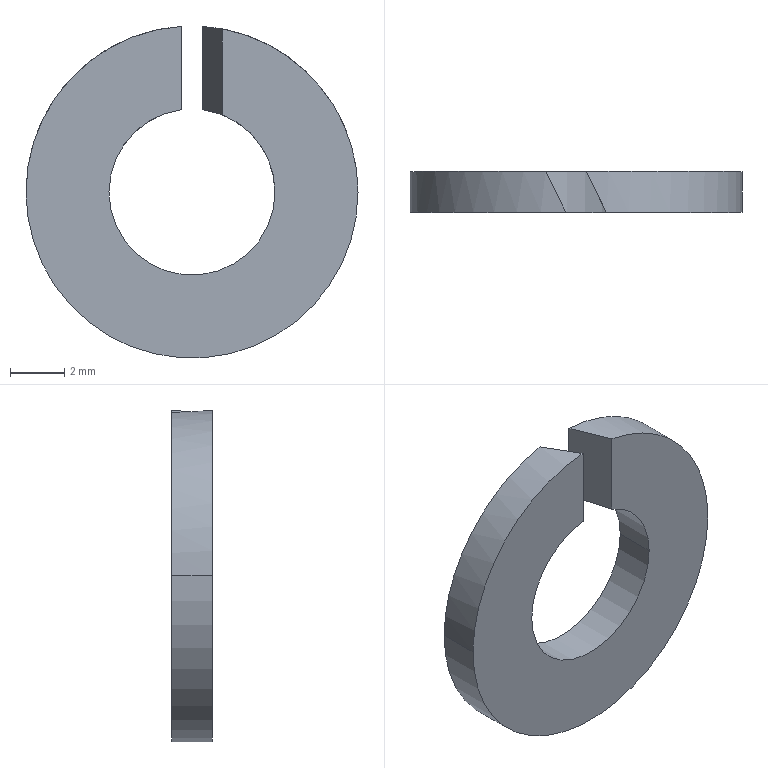Part | STEP file | ZZ24-M6-22 | 1 solid | 10 faces | box 12.2 x 1.5 x 12.188 mm | volume 124.605 mm3 | cylinder 6 | plane 4 | commonest cylinder face diameters 6.1 x3 12.2 x3
STEP:
#1=CARTESIAN_POINT('',(0.,0.,0.));
#2=DIRECTION('',(0.,0.,1.));
#3=DIRECTION('',(1.,0.,0.));
#4=AXIS2_PLACEMENT_3D('',#1,#2,#3);
#5=CARTESIAN_POINT('',(1.116,0.,2.839));
#6=VERTEX_POINT('',#5);
#7=CARTESIAN_POINT('',(0.3842,1.5,3.026));
#8=VERTEX_POINT('',#7);
#9=CARTESIAN_POINT('',(1.116,0.,2.839));
#10=CARTESIAN_POINT('',(0.8803,0.4828,2.931));
#11=CARTESIAN_POINT('',(0.6352,0.9854,2.994));
#12=CARTESIAN_POINT('',(0.3842,1.5,3.026));
#13=(BOUNDED_CURVE()B_SPLINE_CURVE(3,(#9,#10,#11,#12),.UNSPECIFIED.,.F.,.F.)B_SPLINE_CURVE_WITH_KNOTS((4,4),(1.196,1.444),.PIECEWISE_BEZIER_KNOTS.)CURVE()GEOMETRIC_REPRESENTATION_ITEM()RATIONAL_B_SPLINE_CURVE((1.,0.9949,0.9949,1.))REPRESENTATION_ITEM(''));
#14=CARTESIAN_POINT('',(0.,1.5,0.));
#15=DIRECTION('',(0.,-1.,0.));
#16=DIRECTION('',(-1.,0.,0.001512));
#17=AXIS2_PLACEMENT_3D('',#14,#15,#16);
#18=CYLINDRICAL_SURFACE('',#17,3.05);
#19=CARTESIAN_POINT('',(4.339,1.5));
#20=CARTESIAN_POINT('',(4.343,1.478));
#21=CARTESIAN_POINT('',(4.351,1.434));
#22=CARTESIAN_POINT('',(4.362,1.368));
#23=CARTESIAN_POINT('',(4.373,1.302));
#24=CARTESIAN_POINT('',(4.384,1.235));
#25=CARTESIAN_POINT('',(4.396,1.169));
#26=CARTESIAN_POINT('',(4.407,1.101));
#27=CARTESIAN_POINT('',(4.418,1.034));
#28=CARTESIAN_POINT('',(4.43,0.9663));
#29=CARTESIAN_POINT('',(4.441,0.8984));
#30=CARTESIAN_POINT('',(4.452,0.8303));
#31=CARTESIAN_POINT('',(4.463,0.762));
#32=CARTESIAN_POINT('',(4.475,0.6934));
#33=CARTESIAN_POINT('',(4.486,0.6247));
#34=CARTESIAN_POINT('',(4.497,0.5558));
#35=CARTESIAN_POINT('',(4.509,0.4867));
#36=CARTESIAN_POINT('',(4.52,0.4175));
#37=CARTESIAN_POINT('',(4.531,0.3482));
#38=CARTESIAN_POINT('',(4.543,0.2787));
#39=CARTESIAN_POINT('',(4.554,0.2092));
#40=CARTESIAN_POINT('',(4.565,0.1395));
#41=CARTESIAN_POINT('',(4.576,0.0698));
#42=CARTESIAN_POINT('',(4.584,0.02327));
#43=CARTESIAN_POINT('',(4.588,0.));
#44=B_SPLINE_CURVE_WITH_KNOTS('',3,(#19,#20,#21,#22,#23,#24,#25,#26,#27,#28,#29,#30,#31,#32,#33,#34,#35,#36,#37,#38,#39,#40,#41,#42,#43),.UNSPECIFIED.,.F.,.F.,(4,1,1,1,1,1,1,1,1,1,1,1,1,1,1,1,1,1,1,1,1,1,4),(1.196,1.208,1.219,1.23,1.241,1.253,1.264,1.275,1.287,1.298,1.309,1.32,1.332,1.343,1.354,1.366,1.377,1.388,1.399,1.411,1.422,1.433,1.444),.QUASI_UNIFORM_KNOTS.);
#45=(GEOMETRIC_REPRESENTATION_CONTEXT(2)PARAMETRIC_REPRESENTATION_CONTEXT()REPRESENTATION_CONTEXT('',''));
#46=DEFINITIONAL_REPRESENTATION('',(#44),#45);
#47=PCURVE('',#18,#46);
#48=CARTESIAN_POINT('',(1.116,0.,6.1));
#49=DIRECTION('',(-0.8988,-0.4384,0.));
#50=DIRECTION('',(0.4384,-0.8988,0.));
#51=AXIS2_PLACEMENT_3D('',#48,#49,#50);
#52=PLANE('',#51);
#53=CARTESIAN_POINT('',(0.,-3.261));
#54=CARTESIAN_POINT('',(-0.5372,-3.169));
#55=CARTESIAN_POINT('',(-1.096,-3.106));
#56=CARTESIAN_POINT('',(-1.669,-3.074));
#57=(BOUNDED_CURVE()B_SPLINE_CURVE(3,(#53,#54,#55,#56),.UNSPECIFIED.,.F.,.F.)B_SPLINE_CURVE_WITH_KNOTS((4,4),(1.196,1.444),.PIECEWISE_BEZIER_KNOTS.)CURVE()GEOMETRIC_REPRESENTATION_ITEM()RATIONAL_B_SPLINE_CURVE((1.,0.9949,0.9949,1.))REPRESENTATION_ITEM(''));
#58=(GEOMETRIC_REPRESENTATION_CONTEXT(2)PARAMETRIC_REPRESENTATION_CONTEXT()REPRESENTATION_CONTEXT('',''));
#59=DEFINITIONAL_REPRESENTATION('',(#57),#58);
#60=PCURVE('',#52,#59);
#61=SURFACE_CURVE('',#13,(#47,#60),.PCURVE_S1.);
#62=EDGE_CURVE('',#6,#8,#61,.T.);
#63=ORIENTED_EDGE('',*,*,#62,.F.);
#64=CARTESIAN_POINT('',(3.05,0.,-0.004612));
#65=VERTEX_POINT('',#64);
#66=CARTESIAN_POINT('',(0.,0.,0.));
#67=DIRECTION('',(0.,1.,0.));
#68=DIRECTION('',(1.,0.,-0.001512));
#69=AXIS2_PLACEMENT_3D('',#66,#67,#68);
#70=CIRCLE('',#69,3.05);
#71=CARTESIAN_POINT('',(9.425,1.5));
#72=DIRECTION('',(-1.,0.));
#73=VECTOR('',#72,1.);
#74=LINE('',#71,#73);
#75=(GEOMETRIC_REPRESENTATION_CONTEXT(2)PARAMETRIC_REPRESENTATION_CONTEXT()REPRESENTATION_CONTEXT('',''));
#76=DEFINITIONAL_REPRESENTATION('',(#74),#75);
#77=PCURVE('',#18,#76);
#78=CARTESIAN_POINT('',(0.,0.,0.));
#79=DIRECTION('',(0.,-1.,0.));
#80=DIRECTION('',(-1.,0.,0.001512));
#81=AXIS2_PLACEMENT_3D('',#78,#79,#80);
#82=PLANE('',#81);
#83=CARTESIAN_POINT('',(-3.05,0.));
#84=CARTESIAN_POINT('',(-3.05,5.283));
#85=CARTESIAN_POINT('',(1.525,2.641));
#86=CARTESIAN_POINT('',(6.1,0.));
#87=CARTESIAN_POINT('',(1.525,-2.641));
#88=CARTESIAN_POINT('',(-3.05,-5.283));
#89=CARTESIAN_POINT('',(-3.05,0.));
#90=(BOUNDED_CURVE()B_SPLINE_CURVE(2,(#83,#84,#85,#86,#87,#88,#89),.UNSPECIFIED.,.T.,.F.)B_SPLINE_CURVE_WITH_KNOTS((1,2,2,2,2,1),(-2.094,0.,2.094,4.189,6.283,8.378),.UNSPECIFIED.)CURVE()GEOMETRIC_REPRESENTATION_ITEM()RATIONAL_B_SPLINE_CURVE((1.,0.5,1.,0.5,1.,0.5,1.))REPRESENTATION_ITEM(''));
#91=(GEOMETRIC_REPRESENTATION_CONTEXT(2)PARAMETRIC_REPRESENTATION_CONTEXT()REPRESENTATION_CONTEXT('',''));
#92=DEFINITIONAL_REPRESENTATION('',(#90),#91);
#93=PCURVE('',#82,#92);
#94=SURFACE_CURVE('',#70,(#77,#93),.PCURVE_S1.);
#95=EDGE_CURVE('',#6,#65,#94,.T.);
#96=ORIENTED_EDGE('',*,*,#95,.T.);
#97=CARTESIAN_POINT('',(3.05,1.5,-0.004612));
#98=VERTEX_POINT('',#97);
#99=CARTESIAN_POINT('',(3.05,1.5,-0.004612));
#100=DIRECTION('',(0.,-1.,0.));
#101=VECTOR('',#100,1.);
#102=LINE('',#99,#101);
#103=CARTESIAN_POINT('',(3.142,0.));
#104=DIRECTION('',(0.,1.));
#105=VECTOR('',#104,1.);
#106=LINE('',#103,#105);
#107=(GEOMETRIC_REPRESENTATION_CONTEXT(2)PARAMETRIC_REPRESENTATION_CONTEXT()REPRESENTATION_CONTEXT('',''));
#108=DEFINITIONAL_REPRESENTATION('',(#106),#107);
#109=PCURVE('',#18,#108);
#110=CARTESIAN_POINT('',(0.,1.5,0.));
#111=DIRECTION('',(0.,-1.,0.));
#112=DIRECTION('',(-1.,0.,0.001512));
#113=AXIS2_PLACEMENT_3D('',#110,#111,#112);
#114=CYLINDRICAL_SURFACE('',#113,3.05);
#115=CARTESIAN_POINT('',(3.142,0.));
#116=DIRECTION('',(0.,1.));
#117=VECTOR('',#116,1.);
#118=LINE('',#115,#117);
#119=(GEOMETRIC_REPRESENTATION_CONTEXT(2)PARAMETRIC_REPRESENTATION_CONTEXT()REPRESENTATION_CONTEXT('',''));
#120=DEFINITIONAL_REPRESENTATION('',(#118),#119);
#121=PCURVE('',#114,#120);
#122=SURFACE_CURVE('',#102,(#109,#121),.PCURVE_S1.);
#123=EDGE_CURVE('',#98,#65,#122,.T.);
#124=ORIENTED_EDGE('',*,*,#123,.F.);
#125=CARTESIAN_POINT('',(0.,1.5,0.));
#126=DIRECTION('',(0.,-1.,0.));
#127=DIRECTION('',(-1.,0.,0.001512));
#128=AXIS2_PLACEMENT_3D('',#125,#126,#127);
#129=CIRCLE('',#128,3.05);
#130=CARTESIAN_POINT('',(0.,0.));
#131=DIRECTION('',(1.,0.));
#132=VECTOR('',#131,1.);
#133=LINE('',#130,#132);
#134=(GEOMETRIC_REPRESENTATION_CONTEXT(2)PARAMETRIC_REPRESENTATION_CONTEXT()REPRESENTATION_CONTEXT('',''));
#135=DEFINITIONAL_REPRESENTATION('',(#133),#134);
#136=PCURVE('',#18,#135);
#137=CARTESIAN_POINT('',(0.,1.5,0.));
#138=DIRECTION('',(0.,1.,0.));
#139=DIRECTION('',(1.,0.,-0.001512));
#140=AXIS2_PLACEMENT_3D('',#137,#138,#139);
#141=PLANE('',#140);
#142=CARTESIAN_POINT('',(-3.05,0.));
#143=CARTESIAN_POINT('',(-3.05,5.283));
#144=CARTESIAN_POINT('',(1.525,2.641));
#145=CARTESIAN_POINT('',(6.1,0.));
#146=CARTESIAN_POINT('',(1.525,-2.641));
#147=CARTESIAN_POINT('',(-3.05,-5.283));
#148=CARTESIAN_POINT('',(-3.05,0.));
#149=(BOUNDED_CURVE()B_SPLINE_CURVE(2,(#142,#143,#144,#145,#146,#147,#148),.UNSPECIFIED.,.T.,.F.)B_SPLINE_CURVE_WITH_KNOTS((1,2,2,2,2,1),(-2.094,0.,2.094,4.189,6.283,8.378),.UNSPECIFIED.)CURVE()GEOMETRIC_REPRESENTATION_ITEM()RATIONAL_B_SPLINE_CURVE((1.,0.5,1.,0.5,1.,0.5,1.))REPRESENTATION_ITEM(''));
#150=(GEOMETRIC_REPRESENTATION_CONTEXT(2)PARAMETRIC_REPRESENTATION_CONTEXT()REPRESENTATION_CONTEXT('',''));
#151=DEFINITIONAL_REPRESENTATION('',(#149),#150);
#152=PCURVE('',#141,#151);
#153=SURFACE_CURVE('',#129,(#136,#152),.PCURVE_S1.);
#154=EDGE_CURVE('',#98,#8,#153,.T.);
#155=ORIENTED_EDGE('',*,*,#154,.T.);
#156=EDGE_LOOP('',(#63,#96,#124,#155));
#157=FACE_BOUND('',#156,.F.);
#158=ADVANCED_FACE('',(#157),#18,.F.);
#159=CARTESIAN_POINT('',(-3.05,0.,0.004612));
#160=VERTEX_POINT('',#159);
#161=CARTESIAN_POINT('',(0.,0.,0.));
#162=DIRECTION('',(0.,1.,0.));
#163=DIRECTION('',(1.,0.,-0.001512));
#164=AXIS2_PLACEMENT_3D('',#161,#162,#163);
#165=CIRCLE('',#164,3.05);
#166=CARTESIAN_POINT('',(3.142,1.5));
#167=DIRECTION('',(-1.,0.));
#168=VECTOR('',#167,1.);
#169=LINE('',#166,#168);
#170=(GEOMETRIC_REPRESENTATION_CONTEXT(2)PARAMETRIC_REPRESENTATION_CONTEXT()REPRESENTATION_CONTEXT('',''));
#171=DEFINITIONAL_REPRESENTATION('',(#169),#170);
#172=PCURVE('',#114,#171);
#173=CARTESIAN_POINT('',(-3.05,0.));
#174=CARTESIAN_POINT('',(-3.05,5.283));
#175=CARTESIAN_POINT('',(1.525,2.641));
#176=CARTESIAN_POINT('',(6.1,0.));
#177=CARTESIAN_POINT('',(1.525,-2.641));
#178=CARTESIAN_POINT('',(-3.05,-5.283));
#179=CARTESIAN_POINT('',(-3.05,0.));
#180=(BOUNDED_CURVE()B_SPLINE_CURVE(2,(#173,#174,#175,#176,#177,#178,#179),.UNSPECIFIED.,.T.,.F.)B_SPLINE_CURVE_WITH_KNOTS((1,2,2,2,2,1),(-2.094,0.,2.094,4.189,6.283,8.378),.UNSPECIFIED.)CURVE()GEOMETRIC_REPRESENTATION_ITEM()RATIONAL_B_SPLINE_CURVE((1.,0.5,1.,0.5,1.,0.5,1.))REPRESENTATION_ITEM(''));
#181=(GEOMETRIC_REPRESENTATION_CONTEXT(2)PARAMETRIC_REPRESENTATION_CONTEXT()REPRESENTATION_CONTEXT('',''));
#182=DEFINITIONAL_REPRESENTATION('',(#180),#181);
#183=PCURVE('',#82,#182);
#184=SURFACE_CURVE('',#165,(#172,#183),.PCURVE_S1.);
#185=EDGE_CURVE('',#65,#160,#184,.T.);
#186=ORIENTED_EDGE('',*,*,#185,.T.);
#187=CARTESIAN_POINT('',(-3.05,1.5,0.004612));
#188=VERTEX_POINT('',#187);
#189=CARTESIAN_POINT('',(-3.05,1.5,0.004612));
#190=DIRECTION('',(0.,-1.,0.));
#191=VECTOR('',#190,1.);
#192=LINE('',#189,#191);
#193=CARTESIAN_POINT('',(0.,0.));
#194=DIRECTION('',(0.,1.));
#195=VECTOR('',#194,1.);
#196=LINE('',#193,#195);
#197=(GEOMETRIC_REPRESENTATION_CONTEXT(2)PARAMETRIC_REPRESENTATION_CONTEXT()REPRESENTATION_CONTEXT('',''));
#198=DEFINITIONAL_REPRESENTATION('',(#196),#197);
#199=PCURVE('',#114,#198);
#200=CARTESIAN_POINT('',(0.,1.5,0.));
#201=DIRECTION('',(0.,-1.,0.));
#202=DIRECTION('',(-1.,0.,0.001512));
#203=AXIS2_PLACEMENT_3D('',#200,#201,#202);
#204=CYLINDRICAL_SURFACE('',#203,3.05);
#205=CARTESIAN_POINT('',(6.283,0.));
#206=DIRECTION('',(0.,1.));
#207=VECTOR('',#206,1.);
#208=LINE('',#205,#207);
#209=(GEOMETRIC_REPRESENTATION_CONTEXT(2)PARAMETRIC_REPRESENTATION_CONTEXT()REPRESENTATION_CONTEXT('',''));
#210=DEFINITIONAL_REPRESENTATION('',(#208),#209);
#211=PCURVE('',#204,#210);
#212=SURFACE_CURVE('',#192,(#199,#211),.PCURVE_S1.);
#213=EDGE_CURVE('',#188,#160,#212,.T.);
#214=ORIENTED_EDGE('',*,*,#213,.F.);
#215=CARTESIAN_POINT('',(0.,1.5,0.));
#216=DIRECTION('',(0.,-1.,0.));
#217=DIRECTION('',(-1.,0.,0.001512));
#218=AXIS2_PLACEMENT_3D('',#215,#216,#217);
#219=CIRCLE('',#218,3.05);
#220=CARTESIAN_POINT('',(0.,0.));
#221=DIRECTION('',(1.,0.));
#222=VECTOR('',#221,1.);
#223=LINE('',#220,#222);
#224=(GEOMETRIC_REPRESENTATION_CONTEXT(2)PARAMETRIC_REPRESENTATION_CONTEXT()REPRESENTATION_CONTEXT('',''));
#225=DEFINITIONAL_REPRESENTATION('',(#223),#224);
#226=PCURVE('',#114,#225);
#227=CARTESIAN_POINT('',(-3.05,0.));
#228=CARTESIAN_POINT('',(-3.05,5.283));
#229=CARTESIAN_POINT('',(1.525,2.641));
#230=CARTESIAN_POINT('',(6.1,0.));
#231=CARTESIAN_POINT('',(1.525,-2.641));
#232=CARTESIAN_POINT('',(-3.05,-5.283));
#233=CARTESIAN_POINT('',(-3.05,0.));
#234=(BOUNDED_CURVE()B_SPLINE_CURVE(2,(#227,#228,#229,#230,#231,#232,#233),.UNSPECIFIED.,.T.,.F.)B_SPLINE_CURVE_WITH_KNOTS((1,2,2,2,2,1),(-2.094,0.,2.094,4.189,6.283,8.378),.UNSPECIFIED.)CURVE()GEOMETRIC_REPRESENTATION_ITEM()RATIONAL_B_SPLINE_CURVE((1.,0.5,1.,0.5,1.,0.5,1.))REPRESENTATION_ITEM(''));
#235=(GEOMETRIC_REPRESENTATION_CONTEXT(2)PARAMETRIC_REPRESENTATION_CONTEXT()REPRESENTATION_CONTEXT('',''));
#236=DEFINITIONAL_REPRESENTATION('',(#234),#235);
#237=PCURVE('',#141,#236);
#238=SURFACE_CURVE('',#219,(#226,#237),.PCURVE_S1.);
#239=EDGE_CURVE('',#188,#98,#238,.T.);
#240=ORIENTED_EDGE('',*,*,#239,.T.);
#241=ORIENTED_EDGE('',*,*,#123,.T.);
#242=EDGE_LOOP('',(#186,#214,#240,#241));
#243=FACE_BOUND('',#242,.F.);
#244=ADVANCED_FACE('',(#243),#114,.F.);
#245=CARTESIAN_POINT('',(-6.1,1.5,0.009225));
#246=VERTEX_POINT('',#245);
#247=CARTESIAN_POINT('',(6.1,1.5,-0.009225));
#248=VERTEX_POINT('',#247);
#249=CARTESIAN_POINT('',(0.,1.5,0.));
#250=DIRECTION('',(0.,-1.,0.));
#251=DIRECTION('',(-1.,0.,0.001512));
#252=AXIS2_PLACEMENT_3D('',#249,#250,#251);
#253=CIRCLE('',#252,6.1);
#254=CARTESIAN_POINT('',(0.,1.5,0.));
#255=DIRECTION('',(0.,-1.,0.));
#256=DIRECTION('',(-1.,0.,0.001512));
#257=AXIS2_PLACEMENT_3D('',#254,#255,#256);
#258=CYLINDRICAL_SURFACE('',#257,6.1);
#259=CARTESIAN_POINT('',(0.,0.));
#260=DIRECTION('',(1.,0.));
#261=VECTOR('',#260,1.);
#262=LINE('',#259,#261);
#263=(GEOMETRIC_REPRESENTATION_CONTEXT(2)PARAMETRIC_REPRESENTATION_CONTEXT()REPRESENTATION_CONTEXT('',''));
#264=DEFINITIONAL_REPRESENTATION('',(#262),#263);
#265=PCURVE('',#258,#264);
#266=CARTESIAN_POINT('',(-6.1,0.));
#267=CARTESIAN_POINT('',(-6.1,10.566));
#268=CARTESIAN_POINT('',(3.05,5.283));
#269=CARTESIAN_POINT('',(12.2,0.));
#270=CARTESIAN_POINT('',(3.05,-5.283));
#271=CARTESIAN_POINT('',(-6.1,-10.566));
#272=CARTESIAN_POINT('',(-6.1,0.));
#273=(BOUNDED_CURVE()B_SPLINE_CURVE(2,(#266,#267,#268,#269,#270,#271,#272),.UNSPECIFIED.,.T.,.F.)B_SPLINE_CURVE_WITH_KNOTS((1,2,2,2,2,1),(-2.094,0.,2.094,4.189,6.283,8.378),.UNSPECIFIED.)CURVE()GEOMETRIC_REPRESENTATION_ITEM()RATIONAL_B_SPLINE_CURVE((1.,0.5,1.,0.5,1.,0.5,1.))REPRESENTATION_ITEM(''));
#274=(GEOMETRIC_REPRESENTATION_CONTEXT(2)PARAMETRIC_REPRESENTATION_CONTEXT()REPRESENTATION_CONTEXT('',''));
#275=DEFINITIONAL_REPRESENTATION('',(#273),#274);
#276=PCURVE('',#141,#275);
#277=SURFACE_CURVE('',#253,(#265,#276),.PCURVE_S1.);
#278=EDGE_CURVE('',#246,#248,#277,.T.);
#279=ORIENTED_EDGE('',*,*,#278,.T.);
#280=CARTESIAN_POINT('',(6.1,0.,-0.009225));
#281=VERTEX_POINT('',#280);
#282=CARTESIAN_POINT('',(6.1,1.5,-0.009225));
#283=DIRECTION('',(0.,-1.,0.));
#284=VECTOR('',#283,1.);
#285=LINE('',#282,#284);
#286=CARTESIAN_POINT('',(3.142,0.));
#287=DIRECTION('',(0.,1.));
#288=VECTOR('',#287,1.);
#289=LINE('',#286,#288);
#290=(GEOMETRIC_REPRESENTATION_CONTEXT(2)PARAMETRIC_REPRESENTATION_CONTEXT()REPRESENTATION_CONTEXT('',''));
#291=DEFINITIONAL_REPRESENTATION('',(#289),#290);
#292=PCURVE('',#258,#291);
#293=CARTESIAN_POINT('',(0.,1.5,0.));
#294=DIRECTION('',(0.,-1.,0.));
#295=DIRECTION('',(-1.,0.,0.001512));
#296=AXIS2_PLACEMENT_3D('',#293,#294,#295);
#297=CYLINDRICAL_SURFACE('',#296,6.1);
#298=CARTESIAN_POINT('',(3.142,0.));
#299=DIRECTION('',(0.,1.));
#300=VECTOR('',#299,1.);
#301=LINE('',#298,#300);
#302=(GEOMETRIC_REPRESENTATION_CONTEXT(2)PARAMETRIC_REPRESENTATION_CONTEXT()REPRESENTATION_CONTEXT('',''));
#303=DEFINITIONAL_REPRESENTATION('',(#301),#302);
#304=PCURVE('',#297,#303);
#305=SURFACE_CURVE('',#285,(#292,#304),.PCURVE_S1.);
#306=EDGE_CURVE('',#248,#281,#305,.T.);
#307=ORIENTED_EDGE('',*,*,#306,.T.);
#308=CARTESIAN_POINT('',(-6.1,0.,0.009225));
#309=VERTEX_POINT('',#308);
#310=CARTESIAN_POINT('',(0.,0.,0.));
#311=DIRECTION('',(0.,1.,0.));
#312=DIRECTION('',(1.,0.,-0.001512));
#313=AXIS2_PLACEMENT_3D('',#310,#311,#312);
#314=CIRCLE('',#313,6.1);
#315=CARTESIAN_POINT('',(3.142,1.5));
#316=DIRECTION('',(-1.,0.));
#317=VECTOR('',#316,1.);
#318=LINE('',#315,#317);
#319=(GEOMETRIC_REPRESENTATION_CONTEXT(2)PARAMETRIC_REPRESENTATION_CONTEXT()REPRESENTATION_CONTEXT('',''));
#320=DEFINITIONAL_REPRESENTATION('',(#318),#319);
#321=PCURVE('',#258,#320);
#322=CARTESIAN_POINT('',(-6.1,0.));
#323=CARTESIAN_POINT('',(-6.1,10.566));
#324=CARTESIAN_POINT('',(3.05,5.283));
#325=CARTESIAN_POINT('',(12.2,0.));
#326=CARTESIAN_POINT('',(3.05,-5.283));
#327=CARTESIAN_POINT('',(-6.1,-10.566));
#328=CARTESIAN_POINT('',(-6.1,0.));
#329=(BOUNDED_CURVE()B_SPLINE_CURVE(2,(#322,#323,#324,#325,#326,#327,#328),.UNSPECIFIED.,.T.,.F.)B_SPLINE_CURVE_WITH_KNOTS((1,2,2,2,2,1),(-2.094,0.,2.094,4.189,6.283,8.378),.UNSPECIFIED.)CURVE()GEOMETRIC_REPRESENTATION_ITEM()RATIONAL_B_SPLINE_CURVE((1.,0.5,1.,0.5,1.,0.5,1.))REPRESENTATION_ITEM(''));
#330=(GEOMETRIC_REPRESENTATION_CONTEXT(2)PARAMETRIC_REPRESENTATION_CONTEXT()REPRESENTATION_CONTEXT('',''));
#331=DEFINITIONAL_REPRESENTATION('',(#329),#330);
#332=PCURVE('',#82,#331);
#333=SURFACE_CURVE('',#314,(#321,#332),.PCURVE_S1.);
#334=EDGE_CURVE('',#281,#309,#333,.T.);
#335=ORIENTED_EDGE('',*,*,#334,.T.);
#336=CARTESIAN_POINT('',(-6.1,1.5,0.009225));
#337=DIRECTION('',(0.,-1.,0.));
#338=VECTOR('',#337,1.);
#339=LINE('',#336,#338);
#340=CARTESIAN_POINT('',(0.,0.));
#341=DIRECTION('',(0.,1.));
#342=VECTOR('',#341,1.);
#343=LINE('',#340,#342);
#344=(GEOMETRIC_REPRESENTATION_CONTEXT(2)PARAMETRIC_REPRESENTATION_CONTEXT()REPRESENTATION_CONTEXT('',''));
#345=DEFINITIONAL_REPRESENTATION('',(#343),#344);
#346=PCURVE('',#258,#345);
#347=CARTESIAN_POINT('',(0.,1.5,0.));
#348=DIRECTION('',(0.,-1.,0.));
#349=DIRECTION('',(-1.,0.,0.001512));
#350=AXIS2_PLACEMENT_3D('',#347,#348,#349);
#351=CYLINDRICAL_SURFACE('',#350,6.1);
#352=CARTESIAN_POINT('',(6.283,0.));
#353=DIRECTION('',(0.,1.));
#354=VECTOR('',#353,1.);
#355=LINE('',#352,#354);
#356=(GEOMETRIC_REPRESENTATION_CONTEXT(2)PARAMETRIC_REPRESENTATION_CONTEXT()REPRESENTATION_CONTEXT('',''));
#357=DEFINITIONAL_REPRESENTATION('',(#355),#356);
#358=PCURVE('',#351,#357);
#359=SURFACE_CURVE('',#339,(#346,#358),.PCURVE_S1.);
#360=EDGE_CURVE('',#246,#309,#359,.T.);
#361=ORIENTED_EDGE('',*,*,#360,.F.);
#362=EDGE_LOOP('',(#279,#307,#335,#361));
#363=FACE_BOUND('',#362,.T.);
#364=ADVANCED_FACE('',(#363),#258,.T.);
#365=CARTESIAN_POINT('',(-1.116,1.5,5.997));
#366=VERTEX_POINT('',#365);
#367=CARTESIAN_POINT('',(0.,1.5,0.));
#368=DIRECTION('',(0.,-1.,0.));
#369=DIRECTION('',(-1.,0.,0.001512));
#370=AXIS2_PLACEMENT_3D('',#367,#368,#369);
#371=CIRCLE('',#370,6.1);
#372=CARTESIAN_POINT('',(0.,0.));
#373=DIRECTION('',(1.,0.));
#374=VECTOR('',#373,1.);
#375=LINE('',#372,#374);
#376=(GEOMETRIC_REPRESENTATION_CONTEXT(2)PARAMETRIC_REPRESENTATION_CONTEXT()REPRESENTATION_CONTEXT('',''));
#377=DEFINITIONAL_REPRESENTATION('',(#375),#376);
#378=PCURVE('',#351,#377);
#379=CARTESIAN_POINT('',(-6.1,0.));
#380=CARTESIAN_POINT('',(-6.1,10.566));
#381=CARTESIAN_POINT('',(3.05,5.283));
#382=CARTESIAN_POINT('',(12.2,0.));
#383=CARTESIAN_POINT('',(3.05,-5.283));
#384=CARTESIAN_POINT('',(-6.1,-10.566));
#385=CARTESIAN_POINT('',(-6.1,0.));
#386=(BOUNDED_CURVE()B_SPLINE_CURVE(2,(#379,#380,#381,#382,#383,#384,#385),.UNSPECIFIED.,.T.,.F.)B_SPLINE_CURVE_WITH_KNOTS((1,2,2,2,2,1),(-2.094,0.,2.094,4.189,6.283,8.378),.UNSPECIFIED.)CURVE()GEOMETRIC_REPRESENTATION_ITEM()RATIONAL_B_SPLINE_CURVE((1.,0.5,1.,0.5,1.,0.5,1.))REPRESENTATION_ITEM(''));
#387=(GEOMETRIC_REPRESENTATION_CONTEXT(2)PARAMETRIC_REPRESENTATION_CONTEXT()REPRESENTATION_CONTEXT('',''));
#388=DEFINITIONAL_REPRESENTATION('',(#386),#387);
#389=PCURVE('',#141,#388);
#390=SURFACE_CURVE('',#371,(#378,#389),.PCURVE_S1.);
#391=EDGE_CURVE('',#366,#246,#390,.T.);
#392=ORIENTED_EDGE('',*,*,#391,.T.);
#393=ORIENTED_EDGE('',*,*,#360,.T.);
#394=CARTESIAN_POINT('',(-0.3842,0.,6.088));
#395=VERTEX_POINT('',#394);
#396=CARTESIAN_POINT('',(0.,0.,0.));
#397=DIRECTION('',(0.,1.,0.));
#398=DIRECTION('',(1.,0.,-0.001512));
#399=AXIS2_PLACEMENT_3D('',#396,#397,#398);
#400=CIRCLE('',#399,6.1);
#401=CARTESIAN_POINT('',(9.425,1.5));
#402=DIRECTION('',(-1.,0.));
#403=VECTOR('',#402,1.);
#404=LINE('',#401,#403);
#405=(GEOMETRIC_REPRESENTATION_CONTEXT(2)PARAMETRIC_REPRESENTATION_CONTEXT()REPRESENTATION_CONTEXT('',''));
#406=DEFINITIONAL_REPRESENTATION('',(#404),#405);
#407=PCURVE('',#351,#406);
#408=CARTESIAN_POINT('',(-6.1,0.));
#409=CARTESIAN_POINT('',(-6.1,10.566));
#410=CARTESIAN_POINT('',(3.05,5.283));
#411=CARTESIAN_POINT('',(12.2,0.));
#412=CARTESIAN_POINT('',(3.05,-5.283));
#413=CARTESIAN_POINT('',(-6.1,-10.566));
#414=CARTESIAN_POINT('',(-6.1,0.));
#415=(BOUNDED_CURVE()B_SPLINE_CURVE(2,(#408,#409,#410,#411,#412,#413,#414),.UNSPECIFIED.,.T.,.F.)B_SPLINE_CURVE_WITH_KNOTS((1,2,2,2,2,1),(-2.094,0.,2.094,4.189,6.283,8.378),.UNSPECIFIED.)CURVE()GEOMETRIC_REPRESENTATION_ITEM()RATIONAL_B_SPLINE_CURVE((1.,0.5,1.,0.5,1.,0.5,1.))REPRESENTATION_ITEM(''));
#416=(GEOMETRIC_REPRESENTATION_CONTEXT(2)PARAMETRIC_REPRESENTATION_CONTEXT()REPRESENTATION_CONTEXT('',''));
#417=DEFINITIONAL_REPRESENTATION('',(#415),#416);
#418=PCURVE('',#82,#417);
#419=SURFACE_CURVE('',#400,(#407,#418),.PCURVE_S1.);
#420=EDGE_CURVE('',#309,#395,#419,.T.);
#421=ORIENTED_EDGE('',*,*,#420,.T.);
#422=CARTESIAN_POINT('',(-0.3842,0.,6.088));
#423=CARTESIAN_POINT('',(-0.6297,0.5034,6.072));
#424=CARTESIAN_POINT('',(-0.8739,1.004,6.042));
#425=CARTESIAN_POINT('',(-1.116,1.5,5.997));
#426=(BOUNDED_CURVE()B_SPLINE_CURVE(3,(#422,#423,#424,#425),.UNSPECIFIED.,.F.,.F.)B_SPLINE_CURVE_WITH_KNOTS((4,4),(1.634,1.755),.PIECEWISE_BEZIER_KNOTS.)CURVE()GEOMETRIC_REPRESENTATION_ITEM()RATIONAL_B_SPLINE_CURVE((1.,0.9988,0.9988,1.))REPRESENTATION_ITEM(''));
#427=CARTESIAN_POINT('',(4.777,1.5));
#428=CARTESIAN_POINT('',(4.779,1.477));
#429=CARTESIAN_POINT('',(4.782,1.431));
#430=CARTESIAN_POINT('',(4.788,1.363));
#431=CARTESIAN_POINT('',(4.793,1.294));
#432=CARTESIAN_POINT('',(4.799,1.226));
#433=CARTESIAN_POINT('',(4.804,1.157));
#434=CARTESIAN_POINT('',(4.81,1.089));
#435=CARTESIAN_POINT('',(4.815,1.02));
#436=CARTESIAN_POINT('',(4.821,0.9521));
#437=CARTESIAN_POINT('',(4.826,0.8838));
#438=CARTESIAN_POINT('',(4.832,0.8154));
#439=CARTESIAN_POINT('',(4.837,0.7472));
#440=CARTESIAN_POINT('',(4.843,0.679));
#441=CARTESIAN_POINT('',(4.848,0.6108));
#442=CARTESIAN_POINT('',(4.854,0.5427));
#443=CARTESIAN_POINT('',(4.859,0.4746));
#444=CARTESIAN_POINT('',(4.865,0.4066));
#445=CARTESIAN_POINT('',(4.87,0.3387));
#446=CARTESIAN_POINT('',(4.876,0.2708));
#447=CARTESIAN_POINT('',(4.881,0.203));
#448=CARTESIAN_POINT('',(4.887,0.1352));
#449=CARTESIAN_POINT('',(4.892,0.06757));
#450=CARTESIAN_POINT('',(4.896,0.02252));
#451=CARTESIAN_POINT('',(4.898,0.));
#452=B_SPLINE_CURVE_WITH_KNOTS('',3,(#427,#428,#429,#430,#431,#432,#433,#434,#435,#436,#437,#438,#439,#440,#441,#442,#443,#444,#445,#446,#447,#448,#449,#450,#451),.UNSPECIFIED.,.F.,.F.,(4,1,1,1,1,1,1,1,1,1,1,1,1,1,1,1,1,1,1,1,1,1,4),(1.634,1.639,1.645,1.65,1.656,1.661,1.667,1.672,1.678,1.683,1.689,1.694,1.7,1.705,1.711,1.716,1.722,1.727,1.733,1.738,1.744,1.749,1.755),.QUASI_UNIFORM_KNOTS.);
#453=(GEOMETRIC_REPRESENTATION_CONTEXT(2)PARAMETRIC_REPRESENTATION_CONTEXT()REPRESENTATION_CONTEXT('',''));
#454=DEFINITIONAL_REPRESENTATION('',(#452),#453);
#455=PCURVE('',#351,#454);
#456=CARTESIAN_POINT('',(-1.116,1.5,6.1));
#457=DIRECTION('',(0.8988,0.4384,0.));
#458=DIRECTION('',(-0.4384,0.8988,0.));
#459=AXIS2_PLACEMENT_3D('',#456,#457,#458);
#460=PLANE('',#459);
#461=CARTESIAN_POINT('',(-1.669,-0.01211));
#462=CARTESIAN_POINT('',(-1.109,-0.02761));
#463=CARTESIAN_POINT('',(-0.5518,-0.05791));
#464=CARTESIAN_POINT('',(0.,-0.1029));
#465=(BOUNDED_CURVE()B_SPLINE_CURVE(3,(#461,#462,#463,#464),.UNSPECIFIED.,.F.,.F.)B_SPLINE_CURVE_WITH_KNOTS((4,4),(1.634,1.755),.PIECEWISE_BEZIER_KNOTS.)CURVE()GEOMETRIC_REPRESENTATION_ITEM()RATIONAL_B_SPLINE_CURVE((1.,0.9988,0.9988,1.))REPRESENTATION_ITEM(''));
#466=(GEOMETRIC_REPRESENTATION_CONTEXT(2)PARAMETRIC_REPRESENTATION_CONTEXT()REPRESENTATION_CONTEXT('',''));
#467=DEFINITIONAL_REPRESENTATION('',(#465),#466);
#468=PCURVE('',#460,#467);
#469=SURFACE_CURVE('',#426,(#455,#468),.PCURVE_S1.);
#470=EDGE_CURVE('',#395,#366,#469,.T.);
#471=ORIENTED_EDGE('',*,*,#470,.T.);
#472=EDGE_LOOP('',(#392,#393,#421,#471));
#473=FACE_BOUND('',#472,.T.);
#474=ADVANCED_FACE('',(#473),#351,.T.);
#475=CARTESIAN_POINT('',(-0.3842,0.,3.026));
#476=VERTEX_POINT('',#475);
#477=CARTESIAN_POINT('',(-0.3842,0.,6.1));
#478=DIRECTION('',(0.,0.,-1.));
#479=VECTOR('',#478,1.);
#480=LINE('',#477,#479);
#481=CARTESIAN_POINT('',(0.3934,-6.099));
#482=DIRECTION('',(-0.001512,1.));
#483=VECTOR('',#482,1.);
#484=LINE('',#481,#483);
#485=(GEOMETRIC_REPRESENTATION_CONTEXT(2)PARAMETRIC_REPRESENTATION_CONTEXT()REPRESENTATION_CONTEXT('',''));
#486=DEFINITIONAL_REPRESENTATION('',(#484),#485);
#487=PCURVE('',#82,#486);
#488=CARTESIAN_POINT('',(-1.669,0.));
#489=DIRECTION('',(0.,-1.));
#490=VECTOR('',#489,1.);
#491=LINE('',#488,#490);
#492=(GEOMETRIC_REPRESENTATION_CONTEXT(2)PARAMETRIC_REPRESENTATION_CONTEXT()REPRESENTATION_CONTEXT('',''));
#493=DEFINITIONAL_REPRESENTATION('',(#491),#492);
#494=PCURVE('',#460,#493);
#495=SURFACE_CURVE('',#480,(#487,#494),.PCURVE_S1.);
#496=EDGE_CURVE('',#395,#476,#495,.T.);
#497=ORIENTED_EDGE('',*,*,#496,.F.);
#498=ORIENTED_EDGE('',*,*,#420,.F.);
#499=ORIENTED_EDGE('',*,*,#334,.F.);
#500=CARTESIAN_POINT('',(1.116,0.,5.997));
#501=VERTEX_POINT('',#500);
#502=CARTESIAN_POINT('',(0.,0.,0.));
#503=DIRECTION('',(0.,1.,0.));
#504=DIRECTION('',(1.,0.,-0.001512));
#505=AXIS2_PLACEMENT_3D('',#502,#503,#504);
#506=CIRCLE('',#505,6.1);
#507=CARTESIAN_POINT('',(-6.1,0.));
#508=CARTESIAN_POINT('',(-6.1,10.566));
#509=CARTESIAN_POINT('',(3.05,5.283));
#510=CARTESIAN_POINT('',(12.2,0.));
#511=CARTESIAN_POINT('',(3.05,-5.283));
#512=CARTESIAN_POINT('',(-6.1,-10.566));
#513=CARTESIAN_POINT('',(-6.1,0.));
#514=(BOUNDED_CURVE()B_SPLINE_CURVE(2,(#507,#508,#509,#510,#511,#512,#513),.UNSPECIFIED.,.T.,.F.)B_SPLINE_CURVE_WITH_KNOTS((1,2,2,2,2,1),(-2.094,0.,2.094,4.189,6.283,8.378),.UNSPECIFIED.)CURVE()GEOMETRIC_REPRESENTATION_ITEM()RATIONAL_B_SPLINE_CURVE((1.,0.5,1.,0.5,1.,0.5,1.))REPRESENTATION_ITEM(''));
#515=(GEOMETRIC_REPRESENTATION_CONTEXT(2)PARAMETRIC_REPRESENTATION_CONTEXT()REPRESENTATION_CONTEXT('',''));
#516=DEFINITIONAL_REPRESENTATION('',(#514),#515);
#517=PCURVE('',#82,#516);
#518=CARTESIAN_POINT('',(9.425,1.5));
#519=DIRECTION('',(-1.,0.));
#520=VECTOR('',#519,1.);
#521=LINE('',#518,#520);
#522=(GEOMETRIC_REPRESENTATION_CONTEXT(2)PARAMETRIC_REPRESENTATION_CONTEXT()REPRESENTATION_CONTEXT('',''));
#523=DEFINITIONAL_REPRESENTATION('',(#521),#522);
#524=PCURVE('',#297,#523);
#525=SURFACE_CURVE('',#506,(#517,#524),.PCURVE_S1.);
#526=EDGE_CURVE('',#501,#281,#525,.T.);
#527=ORIENTED_EDGE('',*,*,#526,.F.);
#528=CARTESIAN_POINT('',(1.116,0.,6.1));
#529=DIRECTION('',(0.,0.,-1.));
#530=VECTOR('',#529,1.);
#531=LINE('',#528,#530);
#532=CARTESIAN_POINT('',(-1.107,-6.102));
#533=DIRECTION('',(-0.001512,1.));
#534=VECTOR('',#533,1.);
#535=LINE('',#532,#534);
#536=(GEOMETRIC_REPRESENTATION_CONTEXT(2)PARAMETRIC_REPRESENTATION_CONTEXT()REPRESENTATION_CONTEXT('',''));
#537=DEFINITIONAL_REPRESENTATION('',(#535),#536);
#538=PCURVE('',#82,#537);
#539=CARTESIAN_POINT('',(0.,0.));
#540=DIRECTION('',(0.,-1.));
#541=VECTOR('',#540,1.);
#542=LINE('',#539,#541);
#543=(GEOMETRIC_REPRESENTATION_CONTEXT(2)PARAMETRIC_REPRESENTATION_CONTEXT()REPRESENTATION_CONTEXT('',''));
#544=DEFINITIONAL_REPRESENTATION('',(#542),#543);
#545=PCURVE('',#52,#544);
#546=SURFACE_CURVE('',#531,(#538,#545),.PCURVE_S1.);
#547=EDGE_CURVE('',#501,#6,#546,.T.);
#548=ORIENTED_EDGE('',*,*,#547,.T.);
#549=ORIENTED_EDGE('',*,*,#95,.T.);
#550=ORIENTED_EDGE('',*,*,#185,.T.);
#551=CARTESIAN_POINT('',(0.,0.,0.));
#552=DIRECTION('',(0.,1.,0.));
#553=DIRECTION('',(1.,0.,-0.001512));
#554=AXIS2_PLACEMENT_3D('',#551,#552,#553);
#555=CIRCLE('',#554,3.05);
#556=CARTESIAN_POINT('',(-3.05,0.));
#557=CARTESIAN_POINT('',(-3.05,5.283));
#558=CARTESIAN_POINT('',(1.525,2.641));
#559=CARTESIAN_POINT('',(6.1,0.));
#560=CARTESIAN_POINT('',(1.525,-2.641));
#561=CARTESIAN_POINT('',(-3.05,-5.283));
#562=CARTESIAN_POINT('',(-3.05,0.));
#563=(BOUNDED_CURVE()B_SPLINE_CURVE(2,(#556,#557,#558,#559,#560,#561,#562),.UNSPECIFIED.,.T.,.F.)B_SPLINE_CURVE_WITH_KNOTS((1,2,2,2,2,1),(-2.094,0.,2.094,4.189,6.283,8.378),.UNSPECIFIED.)CURVE()GEOMETRIC_REPRESENTATION_ITEM()RATIONAL_B_SPLINE_CURVE((1.,0.5,1.,0.5,1.,0.5,1.))REPRESENTATION_ITEM(''));
#564=(GEOMETRIC_REPRESENTATION_CONTEXT(2)PARAMETRIC_REPRESENTATION_CONTEXT()REPRESENTATION_CONTEXT('',''));
#565=DEFINITIONAL_REPRESENTATION('',(#563),#564);
#566=PCURVE('',#82,#565);
#567=CARTESIAN_POINT('',(9.425,1.5));
#568=DIRECTION('',(-1.,0.));
#569=VECTOR('',#568,1.);
#570=LINE('',#567,#569);
#571=(GEOMETRIC_REPRESENTATION_CONTEXT(2)PARAMETRIC_REPRESENTATION_CONTEXT()REPRESENTATION_CONTEXT('',''));
#572=DEFINITIONAL_REPRESENTATION('',(#570),#571);
#573=PCURVE('',#204,#572);
#574=SURFACE_CURVE('',#555,(#566,#573),.PCURVE_S1.);
#575=EDGE_CURVE('',#160,#476,#574,.T.);
#576=ORIENTED_EDGE('',*,*,#575,.T.);
#577=EDGE_LOOP('',(#497,#498,#499,#527,#548,#549,#550,#576));
#578=FACE_BOUND('',#577,.T.);
#579=ADVANCED_FACE('',(#578),#82,.T.);
#580=CARTESIAN_POINT('',(0.3842,1.5,6.088));
#581=VERTEX_POINT('',#580);
#582=CARTESIAN_POINT('',(0.3842,1.5,6.1));
#583=DIRECTION('',(0.,0.,-1.));
#584=VECTOR('',#583,1.);
#585=LINE('',#582,#584);
#586=CARTESIAN_POINT('',(0.375,-6.101));
#587=DIRECTION('',(0.001512,1.));
#588=VECTOR('',#587,1.);
#589=LINE('',#586,#588);
#590=(GEOMETRIC_REPRESENTATION_CONTEXT(2)PARAMETRIC_REPRESENTATION_CONTEXT()REPRESENTATION_CONTEXT('',''));
#591=DEFINITIONAL_REPRESENTATION('',(#589),#590);
#592=PCURVE('',#141,#591);
#593=CARTESIAN_POINT('',(-1.669,0.));
#594=DIRECTION('',(0.,-1.));
#595=VECTOR('',#594,1.);
#596=LINE('',#593,#595);
#597=(GEOMETRIC_REPRESENTATION_CONTEXT(2)PARAMETRIC_REPRESENTATION_CONTEXT()REPRESENTATION_CONTEXT('',''));
#598=DEFINITIONAL_REPRESENTATION('',(#596),#597);
#599=PCURVE('',#52,#598);
#600=SURFACE_CURVE('',#585,(#592,#599),.PCURVE_S1.);
#601=EDGE_CURVE('',#581,#8,#600,.T.);
#602=ORIENTED_EDGE('',*,*,#601,.F.);
#603=CARTESIAN_POINT('',(0.,1.5,0.));
#604=DIRECTION('',(0.,-1.,0.));
#605=DIRECTION('',(-1.,0.,0.001512));
#606=AXIS2_PLACEMENT_3D('',#603,#604,#605);
#607=CIRCLE('',#606,6.1);
#608=CARTESIAN_POINT('',(-6.1,0.));
#609=CARTESIAN_POINT('',(-6.1,10.566));
#610=CARTESIAN_POINT('',(3.05,5.283));
#611=CARTESIAN_POINT('',(12.2,0.));
#612=CARTESIAN_POINT('',(3.05,-5.283));
#613=CARTESIAN_POINT('',(-6.1,-10.566));
#614=CARTESIAN_POINT('',(-6.1,0.));
#615=(BOUNDED_CURVE()B_SPLINE_CURVE(2,(#608,#609,#610,#611,#612,#613,#614),.UNSPECIFIED.,.T.,.F.)B_SPLINE_CURVE_WITH_KNOTS((1,2,2,2,2,1),(-2.094,0.,2.094,4.189,6.283,8.378),.UNSPECIFIED.)CURVE()GEOMETRIC_REPRESENTATION_ITEM()RATIONAL_B_SPLINE_CURVE((1.,0.5,1.,0.5,1.,0.5,1.))REPRESENTATION_ITEM(''));
#616=(GEOMETRIC_REPRESENTATION_CONTEXT(2)PARAMETRIC_REPRESENTATION_CONTEXT()REPRESENTATION_CONTEXT('',''));
#617=DEFINITIONAL_REPRESENTATION('',(#615),#616);
#618=PCURVE('',#141,#617);
#619=CARTESIAN_POINT('',(0.,0.));
#620=DIRECTION('',(1.,0.));
#621=VECTOR('',#620,1.);
#622=LINE('',#619,#621);
#623=(GEOMETRIC_REPRESENTATION_CONTEXT(2)PARAMETRIC_REPRESENTATION_CONTEXT()REPRESENTATION_CONTEXT('',''));
#624=DEFINITIONAL_REPRESENTATION('',(#622),#623);
#625=PCURVE('',#297,#624);
#626=SURFACE_CURVE('',#607,(#618,#625),.PCURVE_S1.);
#627=EDGE_CURVE('',#248,#581,#626,.T.);
#628=ORIENTED_EDGE('',*,*,#627,.F.);
#629=ORIENTED_EDGE('',*,*,#278,.F.);
#630=ORIENTED_EDGE('',*,*,#391,.F.);
#631=CARTESIAN_POINT('',(-1.116,1.5,2.839));
#632=VERTEX_POINT('',#631);
#633=CARTESIAN_POINT('',(-1.116,1.5,6.1));
#634=DIRECTION('',(0.,0.,-1.));
#635=VECTOR('',#634,1.);
#636=LINE('',#633,#635);
#637=CARTESIAN_POINT('',(-1.125,-6.098));
#638=DIRECTION('',(0.001512,1.));
#639=VECTOR('',#638,1.);
#640=LINE('',#637,#639);
#641=(GEOMETRIC_REPRESENTATION_CONTEXT(2)PARAMETRIC_REPRESENTATION_CONTEXT()REPRESENTATION_CONTEXT('',''));
#642=DEFINITIONAL_REPRESENTATION('',(#640),#641);
#643=PCURVE('',#141,#642);
#644=CARTESIAN_POINT('',(0.,0.));
#645=DIRECTION('',(0.,-1.));
#646=VECTOR('',#645,1.);
#647=LINE('',#644,#646);
#648=(GEOMETRIC_REPRESENTATION_CONTEXT(2)PARAMETRIC_REPRESENTATION_CONTEXT()REPRESENTATION_CONTEXT('',''));
#649=DEFINITIONAL_REPRESENTATION('',(#647),#648);
#650=PCURVE('',#460,#649);
#651=SURFACE_CURVE('',#636,(#643,#650),.PCURVE_S1.);
#652=EDGE_CURVE('',#366,#632,#651,.T.);
#653=ORIENTED_EDGE('',*,*,#652,.T.);
#654=CARTESIAN_POINT('',(0.,1.5,0.));
#655=DIRECTION('',(0.,-1.,0.));
#656=DIRECTION('',(-1.,0.,0.001512));
#657=AXIS2_PLACEMENT_3D('',#654,#655,#656);
#658=CIRCLE('',#657,3.05);
#659=CARTESIAN_POINT('',(-3.05,0.));
#660=CARTESIAN_POINT('',(-3.05,5.283));
#661=CARTESIAN_POINT('',(1.525,2.641));
#662=CARTESIAN_POINT('',(6.1,0.));
#663=CARTESIAN_POINT('',(1.525,-2.641));
#664=CARTESIAN_POINT('',(-3.05,-5.283));
#665=CARTESIAN_POINT('',(-3.05,0.));
#666=(BOUNDED_CURVE()B_SPLINE_CURVE(2,(#659,#660,#661,#662,#663,#664,#665),.UNSPECIFIED.,.T.,.F.)B_SPLINE_CURVE_WITH_KNOTS((1,2,2,2,2,1),(-2.094,0.,2.094,4.189,6.283,8.378),.UNSPECIFIED.)CURVE()GEOMETRIC_REPRESENTATION_ITEM()RATIONAL_B_SPLINE_CURVE((1.,0.5,1.,0.5,1.,0.5,1.))REPRESENTATION_ITEM(''));
#667=(GEOMETRIC_REPRESENTATION_CONTEXT(2)PARAMETRIC_REPRESENTATION_CONTEXT()REPRESENTATION_CONTEXT('',''));
#668=DEFINITIONAL_REPRESENTATION('',(#666),#667);
#669=PCURVE('',#141,#668);
#670=CARTESIAN_POINT('',(0.,0.));
#671=DIRECTION('',(1.,0.));
#672=VECTOR('',#671,1.);
#673=LINE('',#670,#672);
#674=(GEOMETRIC_REPRESENTATION_CONTEXT(2)PARAMETRIC_REPRESENTATION_CONTEXT()REPRESENTATION_CONTEXT('',''));
#675=DEFINITIONAL_REPRESENTATION('',(#673),#674);
#676=PCURVE('',#204,#675);
#677=SURFACE_CURVE('',#658,(#669,#676),.PCURVE_S1.);
#678=EDGE_CURVE('',#632,#188,#677,.T.);
#679=ORIENTED_EDGE('',*,*,#678,.T.);
#680=ORIENTED_EDGE('',*,*,#239,.T.);
#681=ORIENTED_EDGE('',*,*,#154,.T.);
#682=EDGE_LOOP('',(#602,#628,#629,#630,#653,#679,#680,#681));
#683=FACE_BOUND('',#682,.T.);
#684=ADVANCED_FACE('',(#683),#141,.T.);
#685=ORIENTED_EDGE('',*,*,#306,.F.);
#686=ORIENTED_EDGE('',*,*,#627,.T.);
#687=CARTESIAN_POINT('',(0.3842,1.5,6.088));
#688=CARTESIAN_POINT('',(0.6297,0.9966,6.072));
#689=CARTESIAN_POINT('',(0.8739,0.4959,6.042));
#690=CARTESIAN_POINT('',(1.116,0.,5.997));
#691=(BOUNDED_CURVE()B_SPLINE_CURVE(3,(#687,#688,#689,#690),.UNSPECIFIED.,.F.,.F.)B_SPLINE_CURVE_WITH_KNOTS((4,4),(4.775,4.896),.PIECEWISE_BEZIER_KNOTS.)CURVE()GEOMETRIC_REPRESENTATION_ITEM()RATIONAL_B_SPLINE_CURVE((1.,0.9988,0.9988,1.))REPRESENTATION_ITEM(''));
#692=CARTESIAN_POINT('',(4.651,0.));
#693=CARTESIAN_POINT('',(4.649,0.02286));
#694=CARTESIAN_POINT('',(4.645,0.06856));
#695=CARTESIAN_POINT('',(4.64,0.1371));
#696=CARTESIAN_POINT('',(4.634,0.2056));
#697=CARTESIAN_POINT('',(4.629,0.2741));
#698=CARTESIAN_POINT('',(4.623,0.3426));
#699=CARTESIAN_POINT('',(4.618,0.4111));
#700=CARTESIAN_POINT('',(4.612,0.4795));
#701=CARTESIAN_POINT('',(4.607,0.5479));
#702=CARTESIAN_POINT('',(4.601,0.6162));
#703=CARTESIAN_POINT('',(4.596,0.6846));
#704=CARTESIAN_POINT('',(4.59,0.7528));
#705=CARTESIAN_POINT('',(4.585,0.821));
#706=CARTESIAN_POINT('',(4.579,0.8892));
#707=CARTESIAN_POINT('',(4.574,0.9573));
#708=CARTESIAN_POINT('',(4.568,1.025));
#709=CARTESIAN_POINT('',(4.563,1.093));
#710=CARTESIAN_POINT('',(4.557,1.161));
#711=CARTESIAN_POINT('',(4.552,1.229));
#712=CARTESIAN_POINT('',(4.546,1.297));
#713=CARTESIAN_POINT('',(4.541,1.365));
#714=CARTESIAN_POINT('',(4.535,1.432));
#715=CARTESIAN_POINT('',(4.532,1.477));
#716=CARTESIAN_POINT('',(4.53,1.5));
#717=B_SPLINE_CURVE_WITH_KNOTS('',3,(#692,#693,#694,#695,#696,#697,#698,#699,#700,#701,#702,#703,#704,#705,#706,#707,#708,#709,#710,#711,#712,#713,#714,#715,#716),.UNSPECIFIED.,.F.,.F.,(4,1,1,1,1,1,1,1,1,1,1,1,1,1,1,1,1,1,1,1,1,1,4),(4.775,4.781,4.786,4.792,4.797,4.803,4.808,4.814,4.819,4.825,4.83,4.836,4.841,4.847,4.852,4.858,4.863,4.869,4.874,4.88,4.885,4.891,4.896),.QUASI_UNIFORM_KNOTS.);
#718=(GEOMETRIC_REPRESENTATION_CONTEXT(2)PARAMETRIC_REPRESENTATION_CONTEXT()REPRESENTATION_CONTEXT('',''));
#719=DEFINITIONAL_REPRESENTATION('',(#717),#718);
#720=PCURVE('',#297,#719);
#721=CARTESIAN_POINT('',(-1.669,-0.01211));
#722=CARTESIAN_POINT('',(-1.109,-0.02761));
#723=CARTESIAN_POINT('',(-0.5518,-0.05791));
#724=CARTESIAN_POINT('',(0.,-0.1029));
#725=(BOUNDED_CURVE()B_SPLINE_CURVE(3,(#721,#722,#723,#724),.UNSPECIFIED.,.F.,.F.)B_SPLINE_CURVE_WITH_KNOTS((4,4),(4.775,4.896),.PIECEWISE_BEZIER_KNOTS.)CURVE()GEOMETRIC_REPRESENTATION_ITEM()RATIONAL_B_SPLINE_CURVE((1.,0.9988,0.9988,1.))REPRESENTATION_ITEM(''));
#726=(GEOMETRIC_REPRESENTATION_CONTEXT(2)PARAMETRIC_REPRESENTATION_CONTEXT()REPRESENTATION_CONTEXT('',''));
#727=DEFINITIONAL_REPRESENTATION('',(#725),#726);
#728=PCURVE('',#52,#727);
#729=SURFACE_CURVE('',#691,(#720,#728),.PCURVE_S1.);
#730=EDGE_CURVE('',#581,#501,#729,.T.);
#731=ORIENTED_EDGE('',*,*,#730,.T.);
#732=ORIENTED_EDGE('',*,*,#526,.T.);
#733=EDGE_LOOP('',(#685,#686,#731,#732));
#734=FACE_BOUND('',#733,.T.);
#735=ADVANCED_FACE('',(#734),#297,.T.);
#736=ORIENTED_EDGE('',*,*,#601,.T.);
#737=ORIENTED_EDGE('',*,*,#62,.F.);
#738=ORIENTED_EDGE('',*,*,#547,.F.);
#739=ORIENTED_EDGE('',*,*,#730,.F.);
#740=EDGE_LOOP('',(#736,#737,#738,#739));
#741=FACE_BOUND('',#740,.T.);
#742=ADVANCED_FACE('',(#741),#52,.T.);
#743=ORIENTED_EDGE('',*,*,#496,.T.);
#744=CARTESIAN_POINT('',(-1.116,1.5,2.839));
#745=CARTESIAN_POINT('',(-0.8803,1.017,2.931));
#746=CARTESIAN_POINT('',(-0.6352,0.5146,2.994));
#747=CARTESIAN_POINT('',(-0.3842,0.,3.026));
#748=(BOUNDED_CURVE()B_SPLINE_CURVE(3,(#744,#745,#746,#747),.UNSPECIFIED.,.F.,.F.)B_SPLINE_CURVE_WITH_KNOTS((4,4),(4.338,4.586),.PIECEWISE_BEZIER_KNOTS.)CURVE()GEOMETRIC_REPRESENTATION_ITEM()RATIONAL_B_SPLINE_CURVE((1.,0.9949,0.9949,1.))REPRESENTATION_ITEM(''));
#749=CARTESIAN_POINT('',(0.,-3.261));
#750=CARTESIAN_POINT('',(-0.5372,-3.169));
#751=CARTESIAN_POINT('',(-1.096,-3.106));
#752=CARTESIAN_POINT('',(-1.669,-3.074));
#753=(BOUNDED_CURVE()B_SPLINE_CURVE(3,(#749,#750,#751,#752),.UNSPECIFIED.,.F.,.F.)B_SPLINE_CURVE_WITH_KNOTS((4,4),(4.338,4.586),.PIECEWISE_BEZIER_KNOTS.)CURVE()GEOMETRIC_REPRESENTATION_ITEM()RATIONAL_B_SPLINE_CURVE((1.,0.9949,0.9949,1.))REPRESENTATION_ITEM(''));
#754=(GEOMETRIC_REPRESENTATION_CONTEXT(2)PARAMETRIC_REPRESENTATION_CONTEXT()REPRESENTATION_CONTEXT('',''));
#755=DEFINITIONAL_REPRESENTATION('',(#753),#754);
#756=PCURVE('',#460,#755);
#757=CARTESIAN_POINT('',(5.088,0.));
#758=CARTESIAN_POINT('',(5.085,0.02183));
#759=CARTESIAN_POINT('',(5.077,0.06561));
#760=CARTESIAN_POINT('',(5.066,0.1316));
#761=CARTESIAN_POINT('',(5.055,0.1979));
#762=CARTESIAN_POINT('',(5.043,0.2645));
#763=CARTESIAN_POINT('',(5.032,0.3314));
#764=CARTESIAN_POINT('',(5.021,0.3986));
#765=CARTESIAN_POINT('',(5.01,0.466));
#766=CARTESIAN_POINT('',(4.998,0.5337));
#767=CARTESIAN_POINT('',(4.987,0.6016));
#768=CARTESIAN_POINT('',(4.976,0.6697));
#769=CARTESIAN_POINT('',(4.964,0.738));
#770=CARTESIAN_POINT('',(4.953,0.8066));
#771=CARTESIAN_POINT('',(4.942,0.8753));
#772=CARTESIAN_POINT('',(4.93,0.9442));
#773=CARTESIAN_POINT('',(4.919,1.013));
#774=CARTESIAN_POINT('',(4.908,1.082));
#775=CARTESIAN_POINT('',(4.897,1.152));
#776=CARTESIAN_POINT('',(4.885,1.221));
#777=CARTESIAN_POINT('',(4.874,1.291));
#778=CARTESIAN_POINT('',(4.863,1.36));
#779=CARTESIAN_POINT('',(4.851,1.43));
#780=CARTESIAN_POINT('',(4.844,1.477));
#781=CARTESIAN_POINT('',(4.84,1.5));
#782=B_SPLINE_CURVE_WITH_KNOTS('',3,(#757,#758,#759,#760,#761,#762,#763,#764,#765,#766,#767,#768,#769,#770,#771,#772,#773,#774,#775,#776,#777,#778,#779,#780,#781),.UNSPECIFIED.,.F.,.F.,(4,1,1,1,1,1,1,1,1,1,1,1,1,1,1,1,1,1,1,1,1,1,4),(4.338,4.349,4.36,4.372,4.383,4.394,4.406,4.417,4.428,4.439,4.451,4.462,4.473,4.485,4.496,4.507,4.518,4.53,4.541,4.552,4.564,4.575,4.586),.QUASI_UNIFORM_KNOTS.);
#783=(GEOMETRIC_REPRESENTATION_CONTEXT(2)PARAMETRIC_REPRESENTATION_CONTEXT()REPRESENTATION_CONTEXT('',''));
#784=DEFINITIONAL_REPRESENTATION('',(#782),#783);
#785=PCURVE('',#204,#784);
#786=SURFACE_CURVE('',#748,(#756,#785),.PCURVE_S1.);
#787=EDGE_CURVE('',#632,#476,#786,.T.);
#788=ORIENTED_EDGE('',*,*,#787,.F.);
#789=ORIENTED_EDGE('',*,*,#652,.F.);
#790=ORIENTED_EDGE('',*,*,#470,.F.);
#791=EDGE_LOOP('',(#743,#788,#789,#790));
#792=FACE_BOUND('',#791,.T.);
#793=ADVANCED_FACE('',(#792),#460,.T.);
#794=ORIENTED_EDGE('',*,*,#575,.T.);
#795=ORIENTED_EDGE('',*,*,#787,.F.);
#796=ORIENTED_EDGE('',*,*,#678,.T.);
#797=ORIENTED_EDGE('',*,*,#213,.T.);
#798=EDGE_LOOP('',(#794,#795,#796,#797));
#799=FACE_BOUND('',#798,.F.);
#800=ADVANCED_FACE('',(#799),#204,.F.);
#801=CLOSED_SHELL('',(#158,#244,#364,#474,#579,#684,#735,#742,#793,#800));
#802=MANIFOLD_SOLID_BREP('',#801);
#803=(LENGTH_UNIT()NAMED_UNIT(*)SI_UNIT(.MILLI.,.METRE.));
#804=UNCERTAINTY_MEASURE_WITH_UNIT(LENGTH_MEASURE(0.0000001),#803,'','');
#805=(NAMED_UNIT(*)PLANE_ANGLE_UNIT()SI_UNIT($,.RADIAN.));
#806=(NAMED_UNIT(*)SI_UNIT($,.STERADIAN.)SOLID_ANGLE_UNIT());
#807=(GEOMETRIC_REPRESENTATION_CONTEXT(3)GLOBAL_UNCERTAINTY_ASSIGNED_CONTEXT((#804))GLOBAL_UNIT_ASSIGNED_CONTEXT((#803,#805,#806))REPRESENTATION_CONTEXT('',''));
#808=ADVANCED_BREP_SHAPE_REPRESENTATION('',(#4,#802),#807);